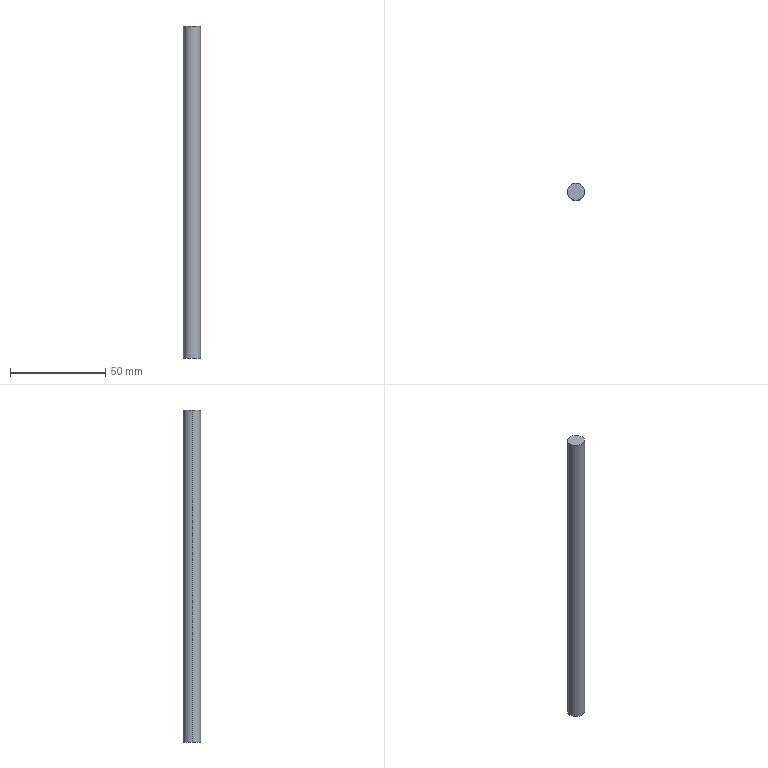Part | SolidWorks | features Extrusion 1 | 1 solid | 4 faces | box 9 x 9 x 174 mm | volume 11069 mm3 | cylinder 2 | plane 2 | commonest cylinder face diameters 9 x2
STEP:
#1=CARTESIAN_POINT('',(4.5,0.,174.));
#2=VERTEX_POINT('',#1);
#3=CARTESIAN_POINT('',(-4.5,0.,174.));
#4=VERTEX_POINT('',#3);
#5=CARTESIAN_POINT('',(0.,0.,174.));
#6=DIRECTION('',(0.,0.,1.));
#7=DIRECTION('',(1.,0.,0.));
#8=AXIS2_PLACEMENT_3D('',#5,#6,#7);
#9=CIRCLE('',#8,4.5);
#10=EDGE_CURVE('',#2,#4,#9,.T.);
#11=ORIENTED_EDGE('',*,*,#10,.F.);
#12=CARTESIAN_POINT('',(4.5,0.,0.));
#13=VERTEX_POINT('',#12);
#14=CARTESIAN_POINT('',(4.5,0.,174.));
#15=DIRECTION('',(0.,0.,-1.));
#16=VECTOR('',#15,1000.);
#17=LINE('',#14,#16);
#18=EDGE_CURVE('',#2,#13,#17,.T.);
#19=ORIENTED_EDGE('',*,*,#18,.T.);
#20=CARTESIAN_POINT('',(-4.5,0.,0.));
#21=VERTEX_POINT('',#20);
#22=CARTESIAN_POINT('',(0.,0.,0.));
#23=DIRECTION('',(0.,0.,1.));
#24=DIRECTION('',(1.,0.,0.));
#25=AXIS2_PLACEMENT_3D('',#22,#23,#24);
#26=CIRCLE('',#25,4.5);
#27=EDGE_CURVE('',#13,#21,#26,.T.);
#28=ORIENTED_EDGE('',*,*,#27,.T.);
#29=CARTESIAN_POINT('',(-4.5,0.,174.));
#30=DIRECTION('',(0.,0.,-1.));
#31=VECTOR('',#30,1000.);
#32=LINE('',#29,#31);
#33=EDGE_CURVE('',#4,#21,#32,.T.);
#34=ORIENTED_EDGE('',*,*,#33,.F.);
#35=EDGE_LOOP('',(#11,#19,#28,#34));
#36=FACE_OUTER_BOUND('',#35,.T.);
#37=CARTESIAN_POINT('',(0.,0.,174.));
#38=DIRECTION('',(0.,0.,-1.));
#39=DIRECTION('',(-1.,0.,0.));
#40=AXIS2_PLACEMENT_3D('',#37,#38,#39);
#41=CYLINDRICAL_SURFACE('',#40,4.5);
#42=ADVANCED_FACE('',(#36),#41,.T.);
#43=ORIENTED_EDGE('',*,*,#18,.F.);
#44=CARTESIAN_POINT('',(0.,0.,174.));
#45=DIRECTION('',(0.,0.,1.));
#46=DIRECTION('',(1.,0.,0.));
#47=AXIS2_PLACEMENT_3D('',#44,#45,#46);
#48=CIRCLE('',#47,4.5);
#49=EDGE_CURVE('',#4,#2,#48,.T.);
#50=ORIENTED_EDGE('',*,*,#49,.F.);
#51=ORIENTED_EDGE('',*,*,#33,.T.);
#52=CARTESIAN_POINT('',(0.,0.,0.));
#53=DIRECTION('',(0.,0.,1.));
#54=DIRECTION('',(1.,0.,0.));
#55=AXIS2_PLACEMENT_3D('',#52,#53,#54);
#56=CIRCLE('',#55,4.5);
#57=EDGE_CURVE('',#21,#13,#56,.T.);
#58=ORIENTED_EDGE('',*,*,#57,.T.);
#59=EDGE_LOOP('',(#43,#50,#51,#58));
#60=FACE_OUTER_BOUND('',#59,.T.);
#61=CARTESIAN_POINT('',(0.,0.,174.));
#62=DIRECTION('',(0.,0.,-1.));
#63=DIRECTION('',(-1.,0.,0.));
#64=AXIS2_PLACEMENT_3D('',#61,#62,#63);
#65=CYLINDRICAL_SURFACE('',#64,4.5);
#66=ADVANCED_FACE('',(#60),#65,.T.);
#67=ORIENTED_EDGE('',*,*,#49,.T.);
#68=ORIENTED_EDGE('',*,*,#10,.T.);
#69=EDGE_LOOP('',(#67,#68));
#70=FACE_OUTER_BOUND('',#69,.T.);
#71=CARTESIAN_POINT('',(0.,0.,174.));
#72=DIRECTION('',(0.,0.,1.));
#73=DIRECTION('',(1.,0.,0.));
#74=AXIS2_PLACEMENT_3D('',#71,#72,#73);
#75=PLANE('',#74);
#76=ADVANCED_FACE('',(#70),#75,.T.);
#77=ORIENTED_EDGE('',*,*,#57,.F.);
#78=ORIENTED_EDGE('',*,*,#27,.F.);
#79=EDGE_LOOP('',(#77,#78));
#80=FACE_OUTER_BOUND('',#79,.T.);
#81=CARTESIAN_POINT('',(0.,0.,0.));
#82=DIRECTION('',(0.,0.,1.));
#83=DIRECTION('',(1.,0.,0.));
#84=AXIS2_PLACEMENT_3D('',#81,#82,#83);
#85=PLANE('',#84);
#86=ADVANCED_FACE('',(#80),#85,.F.);
#87=CLOSED_SHELL('',(#42,#66,#76,#86));
#88=MANIFOLD_SOLID_BREP('',#87);
#89=CARTESIAN_POINT('',(0.,0.,0.));
#90=DIRECTION('',(0.,0.,1.));
#91=DIRECTION('',(1.,0.,0.));
#92=AXIS2_PLACEMENT_3D('',#89,#90,#91);
#93=(LENGTH_UNIT()NAMED_UNIT(*)SI_UNIT(.MILLI.,.METRE.));
#94=UNCERTAINTY_MEASURE_WITH_UNIT(LENGTH_MEASURE(0.00001),#93,'','');
#95=(NAMED_UNIT(*)PLANE_ANGLE_UNIT()SI_UNIT($,.RADIAN.));
#96=(NAMED_UNIT(*)SI_UNIT($,.STERADIAN.)SOLID_ANGLE_UNIT());
#97=(GEOMETRIC_REPRESENTATION_CONTEXT(3)GLOBAL_UNCERTAINTY_ASSIGNED_CONTEXT((#94))GLOBAL_UNIT_ASSIGNED_CONTEXT((#93,#95,#96))REPRESENTATION_CONTEXT('',''));
#98=ADVANCED_BREP_SHAPE_REPRESENTATION('',(#88,#92),#97);